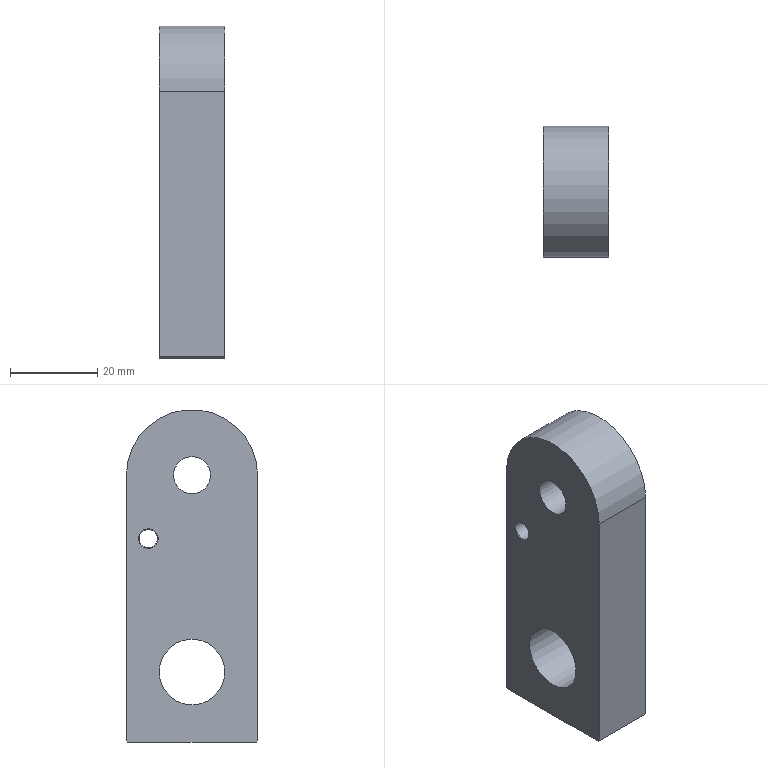NC program | NX | posted with a generic post | part box 15 x 30 x 76 mm
Lines 14638 to 15569 of 31310:
(CURVE_DRIVE_COPY , TOOL : D6R0.5)
N29202 T06 M6
N29204 G53
N29206 G17 G0 G90 X-19.918 Y-1.203 S4000 M3
N29208 G43 Z50. H6
N29210 Z2.994
N29212 G94 G1 Z0.947 F1500.
N29214 Y-1.202 Z0.895
N29216 Y-1.198 Z0.843
N29218 Y-1.192 Z0.791
N29220 Y-1.184 Z0.739
N29222 X-19.919 Y-1.174 Z0.688
N29224 Y-1.161 Z0.637
N29226 Y-1.146 Z0.587
N29228 Y-1.13 Z0.537
N29230 Y-1.11 Z0.488
N29232 X-19.92 Y-1.089 Z0.44
N29234 Y-1.066 Z0.394
N29236 Y-1.041 Z0.348
N29238 X-19.921 Y-1.013 Z0.303
N29240 Y-0.984 Z0.26
N29242 Y-0.953 Z0.217
N29244 X-19.922 Y-0.92 Z0.177
N29246 Y-0.886 Z0.137
N29248 X-19.923 Y-0.849 Z0.1
N29250 Y-0.811 Z0.064
N29252 X-19.924 Y-0.772 Z0.029
N29254 Y-0.731 Z-0.004
N29256 X-19.925 Y-0.689 Z-0.034
N29258 Y-0.645 Z-0.063
N29260 X-19.926 Y-0.6 Z-0.09
N29262 Y-0.554 Z-0.116
N29264 X-19.927 Y-0.507 Z-0.139
N29266 Y-0.459 Z-0.16
N29268 X-19.928 Y-0.411 Z-0.178
N29270 X-19.929 Y-0.361 Z-0.195
N29272 Y-0.311 Z-0.21
N29274 X-19.93 Y-0.26 Z-0.222
N29276 Y-0.208 Z-0.232
N29278 X-19.931 Y-0.157 Z-0.24
N29280 X-19.932 Y-0.105 Z-0.245
N29282 Y-0.052 Z-0.249
N29284 X-19.933 Y0. Z-0.25
N29286 X-19.934 Y0.075
N29288 X-19.937 Y0.15 Z-0.249
N29290 X-19.941 Y0.226 Z-0.25
N29292 X-19.948 Y0.301
N29294 X-19.956 Y0.375
N29296 X-19.966 Y0.45 Z-0.249
N29298 X-19.972 Y0.487 Z-0.25
N29300 X-19.978 Y0.524 Z-0.249
N29302 X-19.992 Y0.598 Z-0.25
N29304 X-20.008 Y0.672
N29306 X-20.025 Y0.745
N29308 X-20.044 Y0.818 Z-0.249
N29310 X-20.065 Y0.89 Z-0.25
N29312 X-20.088 Y0.962
N29314 X-20.112 Y1.033
N29316 X-20.139 Y1.104 Z-0.249
N29318 X-20.166 Y1.174 Z-0.25
N29320 X-20.196 Y1.243
N29322 X-20.227 Y1.311
N29324 X-20.26 Y1.379
N29326 X-20.278 Y1.412
N29328 X-20.295 Y1.446 Z-0.249
N29330 X-20.331 Y1.512 Z-0.25
N29332 X-20.369 Y1.577
N29334 X-20.409 Y1.641
N29336 X-20.45 Y1.704 Z-0.249
N29338 X-20.492 Y1.766 Z-0.25
N29340 X-20.537 Y1.827
N29342 X-20.582 Y1.887
N29344 X-20.629 Y1.946 Z-0.249
N29346 X-20.678 Y2.003 Z-0.25
N29348 X-20.728 Y2.06
N29350 X-20.779 Y2.115
N29352 X-20.831 Y2.169
N29354 X-20.858 Y2.195
N29356 X-20.885 Y2.221 Z-0.249
N29358 X-20.94 Y2.272 Z-0.25
N29360 X-20.997 Y2.322
N29362 X-21.054 Y2.371
N29364 X-21.113 Y2.418 Z-0.249
N29366 X-21.173 Y2.463 Z-0.25
N29368 X-21.234 Y2.508
N29370 X-21.296 Y2.55
N29372 X-21.359 Y2.591 Z-0.249
N29374 X-21.423 Y2.631 Z-0.25
N29376 X-21.488 Y2.669
N29378 X-21.554 Y2.705
N29380 X-21.621 Y2.74
N29382 X-21.655 Y2.756
N29384 X-21.689 Y2.773 Z-0.249
N29386 X-21.757 Y2.804 Z-0.25
N29388 X-21.826 Y2.834
N29390 X-21.896 Y2.861
N29392 X-21.967 Y2.888 Z-0.249
N29394 X-22.038 Y2.912 Z-0.25
N29396 X-22.11 Y2.935
N29398 X-22.182 Y2.956
N29400 X-22.255 Y2.975 Z-0.249
N29402 X-22.328 Y2.992 Z-0.25
N29404 X-22.402 Y3.008
N29406 X-22.476 Y3.022
N29408 X-22.55 Y3.034
N29410 X-22.587 Y3.039
N29412 X-22.625 Y3.044 Z-0.249
N29414 X-22.699 Y3.052 Z-0.25
N29416 X-22.774 Y3.059
N29418 X-22.85 Y3.063
N29420 X-22.925 Y3.066 Z-0.249
N29422 X-23. Y3.067 Z-0.25
N29424 X-23.075 Y3.066
N29426 X-23.15 Y3.063
N29428 X-23.226 Y3.059 Z-0.249
N29430 X-23.301 Y3.052 Z-0.25
N29432 X-23.375 Y3.044
N29434 X-23.45 Y3.034
N29436 X-23.524 Y3.022
N29438 X-23.561 Y3.015
N29440 X-23.598 Y3.008 Z-0.249
N29442 X-23.672 Y2.992 Z-0.25
N29444 X-23.745 Y2.975
N29446 X-23.818 Y2.956
N29448 X-23.89 Y2.935 Z-0.249
N29450 X-23.962 Y2.912 Z-0.25
N29452 X-24.033 Y2.888
N29454 X-24.104 Y2.861
N29456 X-24.174 Y2.834 Z-0.249
N29458 X-24.208 Y2.819 Z-0.25
N29460 X-24.243 Y2.804
N29462 X-24.311 Y2.773
N29464 X-24.379 Y2.74
N29466 X-24.446 Y2.705
N29468 X-24.479 Y2.687
N29470 X-24.512 Y2.669 Z-0.249
N29472 X-24.577 Y2.631 Z-0.25
N29474 X-24.641 Y2.591
N29476 X-24.704 Y2.55
N29478 X-24.766 Y2.508 Z-0.249
N29480 X-24.827 Y2.463 Z-0.25
N29482 X-24.887 Y2.418
N29484 X-24.946 Y2.371
N29486 X-25.003 Y2.322 Z-0.249
N29488 X-25.032 Y2.298 Z-0.25
N29490 X-25.06 Y2.272
N29492 X-25.115 Y2.221
N29494 X-25.169 Y2.169
N29496 X-25.221 Y2.115
N29498 X-25.247 Y2.087
N29500 X-25.272 Y2.06 Z-0.249
N29502 X-25.322 Y2.003 Z-0.25
N29504 X-25.371 Y1.946
N29506 X-25.418 Y1.887
N29508 X-25.463 Y1.827 Z-0.249
N29510 X-25.508 Y1.766 Z-0.25
N29512 X-25.55 Y1.704
N29514 X-25.591 Y1.641
N29516 X-25.631 Y1.577 Z-0.249
N29518 X-25.65 Y1.544 Z-0.25
N29520 X-25.669 Y1.512
N29522 X-25.705 Y1.446
N29524 X-25.74 Y1.379
N29526 X-25.773 Y1.311
N29528 X-25.788 Y1.277
N29530 X-25.804 Y1.243 Z-0.249
N29532 X-25.834 Y1.174 Z-0.25
N29534 X-25.861 Y1.104
N29536 X-25.888 Y1.033
N29538 X-25.912 Y0.962 Z-0.249
N29540 X-25.935 Y0.89 Z-0.25
N29542 X-25.956 Y0.818
N29544 X-25.975 Y0.745
N29546 X-25.992 Y0.672 Z-0.249
N29548 X-26. Y0.635 Z-0.25
N29550 X-26.008 Y0.598
N29552 X-26.022 Y0.524
N29554 X-26.034 Y0.45
N29556 X-26.044 Y0.375
N29558 X-26.048 Y0.338
N29560 X-26.052 Y0.301 Z-0.249
N29562 X-26.059 Y0.226 Z-0.25
N29564 X-26.063 Y0.15
N29566 X-26.066 Y0.075
N29568 X-26.067 Y0. Z-0.249
N29570 X-26.066 Y-0.075 Z-0.25
N29572 X-26.063 Y-0.15
N29574 X-26.059 Y-0.226
N29576 X-26.052 Y-0.301 Z-0.249
N29578 X-26.048 Y-0.338 Z-0.25
N29580 X-26.044 Y-0.375
N29582 X-26.034 Y-0.45
N29584 X-26.022 Y-0.524
N29586 X-26.008 Y-0.598
N29588 X-26. Y-0.635
N29590 X-25.992 Y-0.672 Z-0.249
N29592 X-25.975 Y-0.745 Z-0.25
N29594 X-25.956 Y-0.818
N29596 X-25.935 Y-0.89
N29598 X-25.912 Y-0.962 Z-0.249
N29600 X-25.888 Y-1.033 Z-0.25
N29602 X-25.861 Y-1.104
N29604 X-25.834 Y-1.174
N29606 X-25.804 Y-1.243 Z-0.249
N29608 X-25.788 Y-1.277 Z-0.25
N29610 X-25.773 Y-1.311
N29612 X-25.74 Y-1.379
N29614 X-25.705 Y-1.446
N29616 X-25.669 Y-1.512
N29618 X-25.65 Y-1.544
N29620 X-25.631 Y-1.577 Z-0.249
N29622 X-25.591 Y-1.641 Z-0.25
N29624 X-25.55 Y-1.704
N29626 X-25.508 Y-1.766
N29628 X-25.463 Y-1.827 Z-0.249
N29630 X-25.418 Y-1.887 Z-0.25
N29632 X-25.371 Y-1.946
N29634 X-25.322 Y-2.003
N29636 X-25.272 Y-2.06 Z-0.249
N29638 X-25.247 Y-2.087 Z-0.25
N29640 X-25.221 Y-2.115
N29642 X-25.169 Y-2.169
N29644 X-25.115 Y-2.221
N29646 X-25.06 Y-2.272
N29648 X-25.032 Y-2.298
N29650 X-25.003 Y-2.322 Z-0.249
N29652 X-24.946 Y-2.371 Z-0.25
N29654 X-24.887 Y-2.418
N29656 X-24.827 Y-2.463
N29658 X-24.766 Y-2.508 Z-0.249
N29660 X-24.704 Y-2.55 Z-0.25
N29662 X-24.641 Y-2.591
N29664 X-24.577 Y-2.631
N29666 X-24.512 Y-2.669 Z-0.249
N29668 X-24.479 Y-2.687 Z-0.25
N29670 X-24.446 Y-2.705
N29672 X-24.379 Y-2.74
N29674 X-24.311 Y-2.773
N29676 X-24.243 Y-2.804
N29678 X-24.208 Y-2.819
N29680 X-24.174 Y-2.834 Z-0.249
N29682 X-24.104 Y-2.861 Z-0.25
N29684 X-24.033 Y-2.888
N29686 X-23.962 Y-2.912
N29688 X-23.89 Y-2.935 Z-0.249
N29690 X-23.818 Y-2.956 Z-0.25
N29692 X-23.745 Y-2.975
N29694 X-23.672 Y-2.992
N29696 X-23.598 Y-3.008 Z-0.249
N29698 X-23.561 Y-3.015 Z-0.25
N29700 X-23.524 Y-3.022
N29702 X-23.45 Y-3.034
N29704 X-23.375 Y-3.044
N29706 X-23.301 Y-3.052
N29708 X-23.226 Y-3.059 Z-0.249
N29710 X-23.15 Y-3.063 Z-0.25
N29712 X-23.075 Y-3.066
N29714 X-23. Y-3.067
N29716 X-22.925 Y-3.066 Z-0.249
N29718 X-22.85 Y-3.063 Z-0.25
N29720 X-22.774 Y-3.059
N29722 X-22.699 Y-3.052
N29724 X-22.625 Y-3.044 Z-0.249
N29726 X-22.587 Y-3.039 Z-0.25
N29728 X-22.55 Y-3.034
N29730 X-22.476 Y-3.022
N29732 X-22.402 Y-3.008
N29734 X-22.328 Y-2.992
N29736 X-22.255 Y-2.975 Z-0.249
N29738 X-22.182 Y-2.956 Z-0.25
N29740 X-22.11 Y-2.935
N29742 X-22.038 Y-2.912
N29744 X-21.967 Y-2.888 Z-0.249
N29746 X-21.896 Y-2.861 Z-0.25
N29748 X-21.826 Y-2.834
N29750 X-21.757 Y-2.804
N29752 X-21.689 Y-2.773 Z-0.249
N29754 X-21.655 Y-2.756 Z-0.25
N29756 X-21.621 Y-2.74
N29758 X-21.554 Y-2.705
N29760 X-21.488 Y-2.669
N29762 X-21.423 Y-2.631
N29764 X-21.359 Y-2.591 Z-0.249
N29766 X-21.296 Y-2.55 Z-0.25
N29768 X-21.234 Y-2.508
N29770 X-21.173 Y-2.463
N29772 X-21.113 Y-2.418 Z-0.249
N29774 X-21.054 Y-2.371 Z-0.25
N29776 X-20.997 Y-2.322
N29778 X-20.94 Y-2.272
N29780 X-20.885 Y-2.221 Z-0.249
N29782 X-20.858 Y-2.195 Z-0.25
N29784 X-20.831 Y-2.169
N29786 X-20.779 Y-2.115
N29788 X-20.728 Y-2.06
N29790 X-20.678 Y-2.003
N29792 X-20.629 Y-1.946 Z-0.249
N29794 X-20.582 Y-1.887 Z-0.25
N29796 X-20.537 Y-1.827
N29798 X-20.492 Y-1.766
N29800 X-20.45 Y-1.704 Z-0.249
N29802 X-20.409 Y-1.641 Z-0.25
N29804 X-20.369 Y-1.577
N29806 X-20.331 Y-1.512
N29808 X-20.295 Y-1.446 Z-0.249
N29810 X-20.278 Y-1.412 Z-0.25
N29812 X-20.26 Y-1.379
N29814 X-20.227 Y-1.311
N29816 X-20.196 Y-1.243
N29818 X-20.166 Y-1.174
N29820 X-20.139 Y-1.104 Z-0.249
N29822 X-20.112 Y-1.033 Z-0.25
N29824 X-20.088 Y-0.962
N29826 X-20.065 Y-0.89
N29828 X-20.044 Y-0.818 Z-0.249
N29830 X-20.025 Y-0.745 Z-0.25
N29832 X-20.008 Y-0.672
N29834 X-19.992 Y-0.598
N29836 X-19.978 Y-0.524 Z-0.249
N29838 X-19.972 Y-0.487 Z-0.25
N29840 X-19.966 Y-0.45 Z-0.249
N29842 X-19.956 Y-0.375 Z-0.25
N29844 X-19.948 Y-0.301
N29846 X-19.941 Y-0.226
N29848 X-19.937 Y-0.15 Z-0.249
N29850 X-19.934 Y-0.075 Z-0.25
N29852 X-19.933 Y0.
N29854 X-19.934 Y0.075
N29856 X-19.937 Y0.15
N29858 X-19.942 Y0.226 Z-0.251
N29860 X-19.949 Y0.301
N29862 X-19.957 Y0.375
N29864 X-19.962 Y0.413 Z-0.252
N29866 X-19.967 Y0.45
N29868 X-19.973 Y0.487
N29870 X-19.98 Y0.524
N29872 X-19.994 Y0.598 Z-0.253
N29874 X-20.009 Y0.672
N29876 X-20.027 Y0.745
N29878 X-20.046 Y0.817 Z-0.254
N29880 X-20.068 Y0.89
N29882 X-20.09 Y0.961 Z-0.255
N29884 X-20.103 Y0.997 Z-0.254
N29886 X-20.115 Y1.032 Z-0.255
N29888 X-20.142 Y1.103
N29890 X-20.17 Y1.172
N29892 X-20.199 Y1.241 Z-0.256
N29894 X-20.215 Y1.276
N29896 X-20.223 Y1.293
N29898 X-20.231 Y1.31
N29900 X-20.264 Y1.377 Z-0.257
N29902 X-20.281 Y1.411
N29904 X-20.299 Y1.444
N29906 X-20.335 Y1.51
N29908 X-20.373 Y1.574 Z-0.258
N29910 X-20.413 Y1.638
N29912 X-20.454 Y1.701
N29914 X-20.497 Y1.763 Z-0.259
N29916 X-20.519 Y1.793
N29918 X-20.541 Y1.824
N29920 X-20.587 Y1.883 Z-0.26
N29922 X-20.634 Y1.942
N29924 X-20.682 Y1.999
N29926 X-20.707 Y2.027
N29928 X-20.72 Y2.041 Z-0.261
N29930 X-20.732 Y2.055
N29932 X-20.784 Y2.11
N29934 X-20.836 Y2.164
N29936 X-20.863 Y2.19 Z-0.262
N29938 X-20.89 Y2.216
N29940 X-20.945 Y2.267
N29942 X-21.002 Y2.317 Z-0.263
N29944 X-21.059 Y2.365
N29946 X-21.118 Y2.412
N29948 X-21.178 Y2.457 Z-0.264
N29950 X-21.239 Y2.501
N29952 X-21.301 Y2.543
N29954 X-21.364 Y2.584 Z-0.265
N29956 X-21.396 Y2.604
N29958 X-21.428 Y2.623
N29960 X-21.493 Y2.661 Z-0.266
N29962 X-21.559 Y2.697
N29964 X-21.625 Y2.731
N29966 X-21.659 Y2.747 Z-0.267
N29968 X-21.693 Y2.764
N29970 X-21.761 Y2.795
N29972 X-21.83 Y2.824
N29974 X-21.9 Y2.852 Z-0.268
N29976 X-21.935 Y2.865
N29978 X-21.97 Y2.878
N29980 X-22.041 Y2.902
N29982 X-22.113 Y2.924 Z-0.269
N29984 X-22.185 Y2.945
N29986 X-22.258 Y2.964
N29988 X-22.331 Y2.981 Z-0.27
N29990 X-22.404 Y2.996
N29992 X-22.478 Y3.01 Z-0.271
N29994 X-22.515 Y3.016
N29996 X-22.552 Y3.022
N29998 X-22.589 Y3.027
N30000 X-22.626 Y3.031
N30002 X-22.701 Y3.039 Z-0.272
N30004 X-22.775 Y3.046
N30006 X-22.813 Y3.048
N30008 X-22.831 Y3.049 Z-0.273
N30010 X-22.85 Y3.05 Z-0.272
N30012 X-22.925 Y3.053 Z-0.273
N30014 X-23.
N30016 X-23.075 Y3.052 Z-0.274
N30018 X-23.15 Y3.049
N30020 X-23.225 Y3.044
N30022 X-23.299 Y3.038 Z-0.275
N30024 X-23.374 Y3.029
N30026 X-23.411 Y3.024
N30028 X-23.448 Y3.019 Z-0.276
N30030 X-23.522 Y3.007
N30032 X-23.559 Y3.
N30034 X-23.595 Y2.993
N30036 X-23.669 Y2.977 Z-0.277
N30038 X-23.705 Y2.969
N30040 X-23.723 Y2.964
N30042 X-23.732 Y2.962
N30044 X-23.741 Y2.96
N30046 X-23.814 Y2.94
N30048 X-23.886 Y2.919 Z-0.278
N30050 X-23.957 Y2.897
N30052 X-24.028 Y2.872 Z-0.279
N30054 X-24.098 Y2.846
N30056 X-24.167 Y2.818
N30058 X-24.202 Y2.803
N30060 X-24.236 Y2.788
N30062 X-24.27 Y2.773 Z-0.28
N30064 X-24.304 Y2.757
N30066 X-24.371 Y2.724
N30068 X-24.437 Y2.689 Z-0.281
N30070 X-24.47 Y2.671
N30072 X-24.503 Y2.653
N30074 X-24.535 Y2.634
N30076 X-24.551 Y2.624
N30078 X-24.567 Y2.615
N30080 X-24.631 Y2.575 Z-0.282
N30082 X-24.693 Y2.534
N30084 X-24.755 Y2.492
N30086 X-24.816 Y2.448 Z-0.283
N30088 X-24.875 Y2.403
N30090 X-24.933 Y2.356 Z-0.284
N30092 X-24.99 Y2.307
N30094 X-25.018 Y2.283
N30096 X-25.046 Y2.258
N30098 X-25.101 Y2.207 Z-0.285
N30100 X-25.154 Y2.154
N30102 X-25.206 Y2.101
N30104 X-25.232 Y2.073 Z-0.286
N30106 X-25.257 Y2.046
N30108 X-25.306 Y1.989
N30110 X-25.354 Y1.932 Z-0.287
N30112 X-25.401 Y1.874
N30114 X-25.424 Y1.844
N30116 X-25.446 Y1.814
N30118 X-25.49 Y1.753 Z-0.288
N30120 X-25.532 Y1.692
N30122 X-25.572 Y1.629
N30124 X-25.611 Y1.565 Z-0.289
N30126 X-25.63 Y1.533
N30128 X-25.649 Y1.5
N30130 X-25.684 Y1.435 Z-0.29
N30132 X-25.719 Y1.368
N30134 X-25.735 Y1.335
N30136 X-25.751 Y1.301
N30138 X-25.767 Y1.267 Z-0.291
N30140 X-25.782 Y1.233
N30142 X-25.811 Y1.165
N30144 X-25.839 Y1.095 Z-0.292
N30146 X-25.852 Y1.06
N30148 X-25.858 Y1.043
N30150 X-25.865 Y1.025
N30152 X-25.889 Y0.954
N30154 X-25.911 Y0.883
N30156 X-25.932 Y0.811 Z-0.293
N30158 X-25.951 Y0.739
N30160 X-25.968 Y0.666 Z-0.294
N30162 X-25.976 Y0.63
N30164 X-25.983 Y0.593
N30166 X-25.996 Y0.52
N30168 X-26.002 Y0.483
N30170 X-26.008 Y0.446 Z-0.295
N30172 X-26.018 Y0.372
N30174 X-26.022 Y0.335
N30176 X-26.026 Y0.298
N30178 X-26.032 Y0.224 Z-0.296
N30180 X-26.034 Y0.186
N30182 X-26.035 Y0.168
N30184 X-26.036 Y0.149
N30186 X-26.039 Y0.075 Z-0.297
N30188 X-26.04 Y0.
N30190 X-26.039 Y-0.075
N30192 X-26.036 Y-0.149 Z-0.298
N30194 X-26.031 Y-0.224
N30196 X-26.024 Y-0.298
N30198 X-26.02 Y-0.335 Z-0.299
N30200 X-26.016 Y-0.372
N30202 X-26.005 Y-0.446
N30204 X-25.993 Y-0.519 Z-0.3
N30206 X-25.98 Y-0.593
N30208 X-25.972 Y-0.629
N30210 X-25.964 Y-0.666
N30212 X-25.955 Y-0.702
N30214 X-25.951 Y-0.72
N30216 X-25.946 Y-0.738 Z-0.301
N30218 X-25.927 Y-0.81
N30220 X-25.906 Y-0.882
N30222 X-25.884 Y-0.953 Z-0.302
N30224 X-25.859 Y-1.023
N30226 X-25.833 Y-1.093 Z-0.303
N30228 X-25.805 Y-1.162
N30230 X-25.776 Y-1.23
N30232 X-25.76 Y-1.264 Z-0.304
N30234 X-25.744 Y-1.298
N30236 X-25.711 Y-1.365
N30238 X-25.677 Y-1.431
N30240 X-25.641 Y-1.496 Z-0.305
N30242 X-25.622 Y-1.528
N30244 X-25.603 Y-1.56
N30246 X-25.564 Y-1.624
N30248 X-25.523 Y-1.686 Z-0.306
N30250 X-25.481 Y-1.747
N30252 X-25.459 Y-1.777
N30254 X-25.437 Y-1.807
N30256 X-25.392 Y-1.867 Z-0.307
N30258 X-25.345 Y-1.925
N30260 X-25.297 Y-1.981 Z-0.308
N30262 X-25.272 Y-2.009
N30264 X-25.26 Y-2.023
N30266 X-25.247 Y-2.037
N30268 X-25.222 Y-2.064
N30270 X-25.197 Y-2.091
N30272 X-25.145 Y-2.145 Z-0.309
N30274 X-25.091 Y-2.196
N30276 X-25.064 Y-2.222
N30278 X-25.036 Y-2.247
N30280 X-25.009 Y-2.272 Z-0.31
N30282 X-24.981 Y-2.296
N30284 X-24.923 Y-2.344
N30286 X-24.865 Y-2.39 Z-0.311
N30288 X-24.836 Y-2.413
N30290 X-24.806 Y-2.435
N30292 X-24.745 Y-2.478
N30294 X-24.684 Y-2.52 Z-0.312
N30296 X-24.622 Y-2.561
N30298 X-24.59 Y-2.58
N30300 X-24.574 Y-2.59
N30302 X-24.558 Y-2.599 Z-0.313
N30304 X-24.494 Y-2.637
N30306 X-24.461 Y-2.655
N30308 X-24.428 Y-2.672
N30310 X-24.362 Y-2.706 Z-0.314
N30312 X-24.329 Y-2.723
N30314 X-24.295 Y-2.739
N30316 X-24.228 Y-2.77
N30318 X-24.159 Y-2.799 Z-0.315
N30320 X-24.09 Y-2.826
N30322 X-24.055 Y-2.839
N30324 X-24.038 Y-2.846
N30326 X-24.02 Y-2.852 Z-0.316
N30328 X-23.95 Y-2.876
N30330 X-23.879 Y-2.898
N30332 X-23.808 Y-2.919 Z-0.317
N30334 X-23.736 Y-2.937
N30336 X-23.663 Y-2.954
N30338 X-23.591 Y-2.97 Z-0.318
N30340 X-23.554 Y-2.976
N30342 X-23.518 Y-2.983
N30344 X-23.444 Y-2.994
N30346 X-23.371 Y-3.004 Z-0.319
N30348 X-23.297 Y-3.012
N30350 X-23.223 Y-3.018
N30352 X-23.186 Y-3.021 Z-0.32
N30354 X-23.148 Y-3.023
N30356 X-23.074 Y-3.025
N30358 X-23. Y-3.026 Z-0.321
N30360 X-22.926 Y-3.025
N30362 X-22.852 Y-3.022
N30364 X-22.777 Y-3.017 Z-0.322
N30366 X-22.703 Y-3.011
N30368 X-22.63 Y-3.002
N30370 X-22.593 Y-2.997 Z-0.323
N30372 X-22.556 Y-2.992
N30374 X-22.483 Y-2.98
N30376 X-22.41 Y-2.966 Z-0.324
N30378 X-22.337 Y-2.951
N30380 X-22.301 Y-2.942
N30382 X-22.265 Y-2.933
N30384 X-22.194 Y-2.914 Z-0.325
N30386 X-22.122 Y-2.893
N30388 X-22.052 Y-2.871
N30390 X-22.017 Y-2.859 Z-0.326
N30392 X-21.982 Y-2.846
N30394 X-21.912 Y-2.82
N30396 X-21.843 Y-2.792 Z-0.327
N30398 X-21.775 Y-2.763
N30400 X-21.741 Y-2.748
N30402 X-21.708 Y-2.732
N30404 X-21.674 Y-2.716 Z-0.328
N30406 X-21.641 Y-2.699
N30408 X-21.576 Y-2.665
N30410 X-21.511 Y-2.629
N30412 X-21.447 Y-2.591 Z-0.329
N30414 X-21.384 Y-2.552
N30416 X-21.322 Y-2.512 Z-0.33
N30418 X-21.261 Y-2.47
N30420 X-21.231 Y-2.448
N30422 X-21.201 Y-2.426
N30424 X-21.142 Y-2.381 Z-0.331
N30426 X-21.084 Y-2.334
N30428 X-21.028 Y-2.287
N30430 X-21. Y-2.262
N30432 X-20.986 Y-2.25 Z-0.332
N30434 X-20.972 Y-2.237
N30436 X-20.918 Y-2.187
N30438 X-20.891 Y-2.161
N30440 X-20.865 Y-2.135
N30442 X-20.814 Y-2.082 Z-0.333
N30444 X-20.763 Y-2.027
N30446 X-20.714 Y-1.972 Z-0.334
N30448 X-20.667 Y-1.915
N30450 X-20.621 Y-1.857
N30452 X-20.598 Y-1.827
N30454 X-20.576 Y-1.798 Z-0.335
N30456 X-20.533 Y-1.738
N30458 X-20.491 Y-1.676
N30460 X-20.451 Y-1.614 Z-0.336
N30462 X-20.431 Y-1.583
N30464 X-20.422 Y-1.567
N30466 X-20.412 Y-1.551
N30468 X-20.375 Y-1.487 Z-0.337
N30470 X-20.34 Y-1.422
N30472 X-20.322 Y-1.389
N30474 X-20.306 Y-1.356
N30476 X-20.273 Y-1.29 Z-0.338
N30478 X-20.243 Y-1.222
N30480 X-20.214 Y-1.154
N30482 X-20.187 Y-1.085 Z-0.339
N30484 X-20.161 Y-1.016
N30486 X-20.137 Y-0.946 Z-0.34
N30488 X-20.115 Y-0.875
N30490 X-20.095 Y-0.804
N30492 X-20.085 Y-0.768 Z-0.341
N30494 X-20.08 Y-0.75 Z-0.34
N30496 X-20.076 Y-0.732 Z-0.341
N30498 X-20.059 Y-0.66
N30500 X-20.044 Y-0.588
N30502 X-20.031 Y-0.515 Z-0.342
N30504 X-20.025 Y-0.479
N30506 X-20.019 Y-0.442
N30508 X-20.009 Y-0.369
N30510 X-20.001 Y-0.295 Z-0.343
N30512 X-19.995 Y-0.222
N30514 X-19.993 Y-0.185
N30516 X-19.991 Y-0.148
N30518 X-19.988 Y-0.074 Z-0.344
N30520 Y0.
N30522 X-19.989 Y0.074 Z-0.345
N30524 X-19.992 Y0.148
N30526 X-19.996 Y0.222
N30528 X-20.003 Y0.295 Z-0.346
N30530 X-20.011 Y0.369
N30532 X-20.016 Y0.405
N30534 X-20.022 Y0.442
N30536 X-20.027 Y0.478 Z-0.347
N30538 X-20.033 Y0.515
N30540 X-20.047 Y0.587
N30542 X-20.063 Y0.66 Z-0.348
N30544 X-20.08 Y0.731
N30546 X-20.099 Y0.803
N30548 X-20.12 Y0.874 Z-0.349
N30550 X-20.142 Y0.944
N30552 X-20.154 Y0.979
N30554 X-20.167 Y1.014
N30556 X-20.192 Y1.083 Z-0.35
N30558 X-20.22 Y1.151
N30560 X-20.249 Y1.219
N30562 X-20.265 Y1.253
N30564 X-20.272 Y1.27 Z-0.351
N30566 X-20.28 Y1.286
N30568 X-20.313 Y1.353
N30570 X-20.33 Y1.385
N30572 X-20.347 Y1.418
N30574 X-20.383 Y1.483 Z-0.352
N30576 X-20.42 Y1.546
N30578 X-20.459 Y1.609
N30580 X-20.499 Y1.671 Z-0.353
N30582 X-20.541 Y1.732
N30584 X-20.563 Y1.762
N30586 X-20.585 Y1.791 Z-0.354
N30588 X-20.63 Y1.85
N30590 X-20.676 Y1.907
N30592 X-20.724 Y1.964 Z-0.355
N30594 X-20.748 Y1.991
N30596 X-20.76 Y2.005
N30598 X-20.773 Y2.019
N30600 X-20.823 Y2.073
N30602 X-20.875 Y2.125 Z-0.356
N30604 X-20.901 Y2.151
N30606 X-20.928 Y2.177
N30608 X-20.982 Y2.227 Z-0.357
N30610 X-21.037 Y2.275
N30612 X-21.094 Y2.323
N30614 X-21.151 Y2.369
N30616 X-21.21 Y2.413 Z-0.358
N30618 X-21.27 Y2.456
N30620 X-21.331 Y2.498 Z-0.359
N30622 X-21.393 Y2.538
N30624 X-21.424 Y2.557
N30626 X-21.456 Y2.576
N30628 X-21.52 Y2.613 Z-0.36
N30630 X-21.584 Y2.649
N30632 X-21.65 Y2.682
N30634 X-21.683 Y2.699 Z-0.361
N30636 X-21.716 Y2.714
N30638 X-21.783 Y2.745
N30640 X-21.851 Y2.774 Z-0.362
N30642 X-21.92 Y2.801
N30644 X-21.954 Y2.814
N30646 X-21.989 Y2.826
N30648 X-22.058 Y2.85 Z-0.363
N30650 X-22.129 Y2.872
N30652 X-22.2 Y2.893
N30654 X-22.271 Y2.911 Z-0.364
N30656 X-22.342 Y2.928
N30658 X-22.415 Y2.943
N30660 X-22.487 Y2.956 Z-0.365
N30662 X-22.523 Y2.962
N30664 X-22.56 Y2.968
N30666 X-22.596 Y2.973
N30668 X-22.633 Y2.978
N30670 X-22.706 Y2.985 Z-0.366
N30672 X-22.779 Y2.992
N30674 X-22.816 Y2.994
N30676 X-22.834 Y2.995 Z-0.367
N30678 X-22.853 Y2.996 Z-0.366
N30680 X-22.926 Y2.998 Z-0.367
N30682 X-23. Y2.999
N30684 X-23.074 Y2.998 Z-0.368
N30686 X-23.147 Y2.995
N30688 X-23.221 Y2.99
N30690 X-23.294 Y2.984 Z-0.369
N30692 X-23.367 Y2.975
N30694 X-23.403 Y2.971
N30696 X-23.44 Y2.965
N30698 X-23.512 Y2.953 Z-0.37
N30700 X-23.549 Y2.947
N30702 X-23.585 Y2.94
N30704 X-23.657 Y2.924
N30706 X-23.693 Y2.916 Z-0.371
N30708 X-23.71 Y2.912
N30710 X-23.719 Y2.909
N30712 X-23.728 Y2.907
N30714 X-23.799 Y2.888
N30716 X-23.87 Y2.868
N30718 X-23.94 Y2.845 Z-0.372
N30720 X-24.009 Y2.821
N30722 X-24.078 Y2.795 Z-0.373
N30724 X-24.146 Y2.768
N30726 X-24.214 Y2.739
N30728 X-24.247 Y2.723
N30730 X-24.281 Y2.708 Z-0.374
N30732 X-24.347 Y2.675
N30734 X-24.412 Y2.641
N30736 X-24.444 Y2.624 Z-0.375
N30738 X-24.476 Y2.606
N30740 X-24.508 Y2.587
N30742 X-24.524 Y2.578
N30744 X-24.539 Y2.568
N30746 X-24.602 Y2.53 Z-0.376
N30748 X-24.663 Y2.489
N30750 X-24.724 Y2.448
N30752 X-24.783 Y2.405 Z-0.377
N30754 X-24.842 Y2.36
N30756 X-24.899 Y2.314
N30758 X-24.955 Y2.266 Z-0.378
N30760 X-24.983 Y2.242
N30762 X-25.01 Y2.218
N30764 X-25.064 Y2.167
N30766 X-25.116 Y2.116 Z-0.379
N30768 X-25.167 Y2.063
N30770 X-25.192 Y2.036
N30772 X-25.217 Y2.009
N30774 X-25.265 Y1.954 Z-0.38
N30776 X-25.313 Y1.898
N30778 X-25.358 Y1.84
N30780 X-25.381 Y1.811 Z-0.381
N30782 X-25.403 Y1.782
N30784 X-25.445 Y1.722
N30786 X-25.487 Y1.662 Z-0.382
N30788 X-25.527 Y1.6
N30790 X-25.565 Y1.537
N30792 X-25.584 Y1.506 Z-0.383
N30794 X-25.602 Y1.474
N30796 X-25.637 Y1.409
N30798 X-25.671 Y1.344
N30800 X-25.687 Y1.311 Z-0.384
N30802 X-25.703 Y1.278
N30804 X-25.718 Y1.245
N30806 X-25.733 Y1.211
N30808 X-25.762 Y1.144
N30810 X-25.789 Y1.076 Z-0.385
N30812 X-25.802 Y1.041
N30814 X-25.808 Y1.024
N30816 X-25.814 Y1.007
N30818 X-25.838 Y0.937
N30820 X-25.86 Y0.867 Z-0.386
N30822 X-25.88 Y0.797
N30824 X-25.898 Y0.726 Z-0.387
N30826 X-25.915 Y0.655
N30828 X-25.93 Y0.583
N30830 X-25.943 Y0.511 Z-0.388
N30832 X-25.949 Y0.475
N30834 X-25.955 Y0.438
N30836 X-25.964 Y0.366
N30838 X-25.969 Y0.329 Z-0.389
N30840 X-25.972 Y0.293
N30842 X-25.978 Y0.22
N30844 X-25.981 Y0.183
N30846 X-25.982 Y0.165
N30848 X-25.983 Y0.147 Z-0.39
N30850 X-25.985 Y0.073
N30852 X-25.986 Y0.
N30854 X-25.985 Y-0.073 Z-0.391
N30856 X-25.982 Y-0.146
N30858 X-25.977 Y-0.22
N30860 X-25.971 Y-0.293 Z-0.392
N30862 X-25.967 Y-0.329
N30864 X-25.962 Y-0.365
N30866 X-25.958 Y-0.402
N30868 X-25.952 Y-0.438
N30870 X-25.94 Y-0.51 Z-0.393
N30872 X-25.927 Y-0.582
N30874 X-25.911 Y-0.654
N30876 X-25.903 Y-0.689 Z-0.394
N30878 X-25.899 Y-0.707
N30880 X-25.894 Y-0.725
N30882 X-25.875 Y-0.796
N30884 X-25.855 Y-0.866
N30886 X-25.833 Y-0.936 Z-0.395
N30888 X-25.809 Y-1.005
N30890 X-25.783 Y-1.073 Z-0.396
N30892 X-25.755 Y-1.141
N30894 X-25.726 Y-1.209
N30896 X-25.711 Y-1.242 Z-0.397
N30898 X-25.696 Y-1.275
N30900 X-25.663 Y-1.341
N30902 X-25.63 Y-1.406
N30904 X-25.594 Y-1.47 Z-0.398
N30906 X-25.576 Y-1.501
N30908 X-25.557 Y-1.533
N30910 X-25.519 Y-1.595
N30912 X-25.478 Y-1.656 Z-0.399
N30914 X-25.437 Y-1.716
N30916 X-25.416 Y-1.746
N30918 X-25.394 Y-1.775
N30920 X-25.349 Y-1.834 Z-0.4
N30922 X-25.304 Y-1.891
N30924 X-25.256 Y-1.946 Z-0.401
N30926 X-25.232 Y-1.974
N30928 X-25.22 Y-1.987
N30930 X-25.208 Y-2.001
N30932 X-25.183 Y-2.028
N30934 X-25.158 Y-2.054
N30936 X-25.107 Y-2.107 Z-0.402
N30938 X-25.054 Y-2.158
N30940 X-25.027 Y-2.182
N30942 X-25. Y-2.207
N30944 X-24.946 Y-2.255 Z-0.403
N30946 X-24.889 Y-2.302
N30948 X-24.832 Y-2.348 Z-0.404
N30950 X-24.803 Y-2.37
N30952 X-24.774 Y-2.392
N30954 X-24.715 Y-2.435
N30956 X-24.654 Y-2.476
N30958 X-24.593 Y-2.515 Z-0.405
N30960 X-24.562 Y-2.535
N30962 X-24.546 Y-2.544
N30964 X-24.531 Y-2.554
N30966 X-24.467 Y-2.59 Z-0.406
N30968 X-24.435 Y-2.608
N30970 X-24.403 Y-2.625
N30972 X-24.338 Y-2.659
N30974 X-24.305 Y-2.675
N30976 X-24.273 Y-2.691 Z-0.407
N30978 X-24.206 Y-2.721
N30980 X-24.139 Y-2.749
N30982 X-24.071 Y-2.776 Z-0.408
N30984 X-24.037 Y-2.789
N30986 X-24.02 Y-2.795
N30988 X-24.002 Y-2.802
N30990 X-23.933 Y-2.825
N30992 X-23.864 Y-2.847 Z-0.409
N30994 X-23.793 Y-2.867
N30996 X-23.723 Y-2.885 Z-0.41
N30998 X-23.652 Y-2.902
N31000 X-23.58 Y-2.917
N31002 X-23.544 Y-2.924 Z-0.411
N31004 X-23.508 Y-2.93
N31006 X-23.436 Y-2.942
N31008 X-23.364 Y-2.951
N31010 X-23.291 Y-2.959 Z-0.412
N31012 X-23.219 Y-2.965
N31014 X-23.182 Y-2.967
N31016 X-23.146 Y-2.969
N31018 X-23.073 Y-2.972 Z-0.413
N31020 X-23. Y-2.973
N31022 X-22.927 Y-2.971
N31024 X-22.854 Y-2.969 Z-0.414
N31026 X-22.781 Y-2.964
N31028 X-22.709 Y-2.957 Z-0.415
N31030 X-22.636 Y-2.949
N31032 X-22.6 Y-2.944
N31034 X-22.564 Y-2.939
N31036 X-22.492 Y-2.927 Z-0.416
N31038 X-22.42 Y-2.914
N31040 X-22.349 Y-2.899
N31042 X-22.314 Y-2.89 Z-0.417
N31044 X-22.278 Y-2.881
N31046 X-22.208 Y-2.863
N31048 X-22.138 Y-2.842 Z-0.418
N31050 X-22.068 Y-2.82
N31052 X-22.034 Y-2.808
N31054 X-22. Y-2.796
N31056 X-21.931 Y-2.77
N31058 X-21.864 Y-2.743 Z-0.419